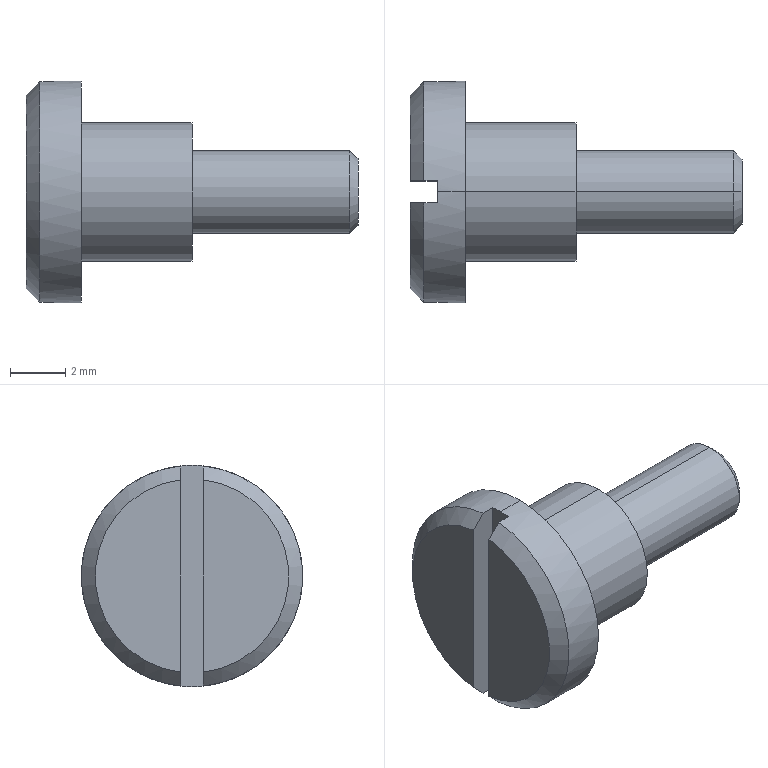Part | STEP file | 0246_012_CBD5-4 | 1 solid | 18 faces | box 12 x 8 x 8 mm | volume 211.87 mm3 | plane 8 | cylinder 6 | cone 4 | commonest cylinder face diameters 3 x2 5 x2 8 x2
STEP:
#1=CARTESIAN_POINT('',(0.,0.,0.));
#2=DIRECTION('',(0.,0.,1.));
#3=DIRECTION('',(1.,0.,0.));
#4=AXIS2_PLACEMENT_3D('',#1,#2,#3);
#5=CARTESIAN_POINT('',(0.,0.,-2.5));
#6=VERTEX_POINT('',#5);
#7=CARTESIAN_POINT('',(0.,0.,2.5));
#8=VERTEX_POINT('',#7);
#9=CARTESIAN_POINT('',(0.,0.,0.));
#10=DIRECTION('',(1.,0.,0.));
#11=DIRECTION('',(0.,0.,-1.));
#12=AXIS2_PLACEMENT_3D('',#9,#10,#11);
#13=CIRCLE('',#12,2.5);
#14=CARTESIAN_POINT('',(2.,0.,0.));
#15=DIRECTION('',(1.,0.,0.));
#16=DIRECTION('',(0.,0.,-1.));
#17=AXIS2_PLACEMENT_3D('',#14,#15,#16);
#18=CYLINDRICAL_SURFACE('',#17,2.5);
#19=CARTESIAN_POINT('',(0.,-2.));
#20=DIRECTION('',(1.,0.));
#21=VECTOR('',#20,1.);
#22=LINE('',#19,#21);
#23=(GEOMETRIC_REPRESENTATION_CONTEXT(2)PARAMETRIC_REPRESENTATION_CONTEXT()REPRESENTATION_CONTEXT('',''));
#24=DEFINITIONAL_REPRESENTATION('',(#22),#23);
#25=PCURVE('',#18,#24);
#26=CARTESIAN_POINT('',(0.,3.25,0.));
#27=DIRECTION('',(1.,0.,0.));
#28=DIRECTION('',(0.,0.,-1.));
#29=AXIS2_PLACEMENT_3D('',#26,#27,#28);
#30=PLANE('',#29);
#31=CARTESIAN_POINT('',(0.,-3.25));
#32=DIRECTION('',(1.,0.));
#33=AXIS2_PLACEMENT_2D('',#31,#32);
#34=CIRCLE('',#33,2.5);
#35=(GEOMETRIC_REPRESENTATION_CONTEXT(2)PARAMETRIC_REPRESENTATION_CONTEXT()REPRESENTATION_CONTEXT('',''));
#36=DEFINITIONAL_REPRESENTATION('',(#34),#35);
#37=PCURVE('',#30,#36);
#38=SURFACE_CURVE('',#13,(#25,#37),.PCURVE_S1.);
#39=EDGE_CURVE('',#6,#8,#38,.T.);
#40=ORIENTED_EDGE('',*,*,#39,.T.);
#41=CARTESIAN_POINT('',(4.,0.,2.5));
#42=VERTEX_POINT('',#41);
#43=CARTESIAN_POINT('',(2.,0.,2.5));
#44=DIRECTION('',(1.,0.,0.));
#45=VECTOR('',#44,1.);
#46=LINE('',#43,#45);
#47=CARTESIAN_POINT('',(3.142,0.));
#48=DIRECTION('',(0.,1.));
#49=VECTOR('',#48,1.);
#50=LINE('',#47,#49);
#51=(GEOMETRIC_REPRESENTATION_CONTEXT(2)PARAMETRIC_REPRESENTATION_CONTEXT()REPRESENTATION_CONTEXT('',''));
#52=DEFINITIONAL_REPRESENTATION('',(#50),#51);
#53=PCURVE('',#18,#52);
#54=CARTESIAN_POINT('',(2.,0.,0.));
#55=DIRECTION('',(1.,0.,0.));
#56=DIRECTION('',(0.,0.,-1.));
#57=AXIS2_PLACEMENT_3D('',#54,#55,#56);
#58=CYLINDRICAL_SURFACE('',#57,2.5);
#59=CARTESIAN_POINT('',(3.142,0.));
#60=DIRECTION('',(0.,1.));
#61=VECTOR('',#60,1.);
#62=LINE('',#59,#61);
#63=(GEOMETRIC_REPRESENTATION_CONTEXT(2)PARAMETRIC_REPRESENTATION_CONTEXT()REPRESENTATION_CONTEXT('',''));
#64=DEFINITIONAL_REPRESENTATION('',(#62),#63);
#65=PCURVE('',#58,#64);
#66=SURFACE_CURVE('',#46,(#53,#65),.PCURVE_S1.);
#67=EDGE_CURVE('',#8,#42,#66,.T.);
#68=ORIENTED_EDGE('',*,*,#67,.T.);
#69=CARTESIAN_POINT('',(4.,0.,-2.5));
#70=VERTEX_POINT('',#69);
#71=CARTESIAN_POINT('',(4.,0.,0.));
#72=DIRECTION('',(-1.,0.,0.));
#73=DIRECTION('',(0.,0.,-1.));
#74=AXIS2_PLACEMENT_3D('',#71,#72,#73);
#75=CIRCLE('',#74,2.5);
#76=CARTESIAN_POINT('',(6.283,2.));
#77=DIRECTION('',(-1.,0.));
#78=VECTOR('',#77,1.);
#79=LINE('',#76,#78);
#80=(GEOMETRIC_REPRESENTATION_CONTEXT(2)PARAMETRIC_REPRESENTATION_CONTEXT()REPRESENTATION_CONTEXT('',''));
#81=DEFINITIONAL_REPRESENTATION('',(#79),#80);
#82=PCURVE('',#18,#81);
#83=CARTESIAN_POINT('',(4.,2.,0.));
#84=DIRECTION('',(1.,0.,0.));
#85=DIRECTION('',(0.,0.,-1.));
#86=AXIS2_PLACEMENT_3D('',#83,#84,#85);
#87=PLANE('',#86);
#88=CARTESIAN_POINT('',(2.5,-2.));
#89=CARTESIAN_POINT('',(2.5,-6.33));
#90=CARTESIAN_POINT('',(-1.25,-4.165));
#91=CARTESIAN_POINT('',(-5.,-2.));
#92=CARTESIAN_POINT('',(-1.25,0.1651));
#93=CARTESIAN_POINT('',(2.5,2.33));
#94=CARTESIAN_POINT('',(2.5,-2.));
#95=(BOUNDED_CURVE()B_SPLINE_CURVE(2,(#88,#89,#90,#91,#92,#93,#94),.UNSPECIFIED.,.T.,.F.)B_SPLINE_CURVE_WITH_KNOTS((1,2,2,2,2,1),(-2.094,0.,2.094,4.189,6.283,8.378),.UNSPECIFIED.)CURVE()GEOMETRIC_REPRESENTATION_ITEM()RATIONAL_B_SPLINE_CURVE((1.,0.5,1.,0.5,1.,0.5,1.))REPRESENTATION_ITEM(''));
#96=(GEOMETRIC_REPRESENTATION_CONTEXT(2)PARAMETRIC_REPRESENTATION_CONTEXT()REPRESENTATION_CONTEXT('',''));
#97=DEFINITIONAL_REPRESENTATION('',(#95),#96);
#98=PCURVE('',#87,#97);
#99=SURFACE_CURVE('',#75,(#82,#98),.PCURVE_S1.);
#100=EDGE_CURVE('',#42,#70,#99,.T.);
#101=ORIENTED_EDGE('',*,*,#100,.T.);
#102=CARTESIAN_POINT('',(2.,0.,-2.5));
#103=DIRECTION('',(1.,0.,0.));
#104=VECTOR('',#103,1.);
#105=LINE('',#102,#104);
#106=CARTESIAN_POINT('',(0.,0.));
#107=DIRECTION('',(0.,1.));
#108=VECTOR('',#107,1.);
#109=LINE('',#106,#108);
#110=(GEOMETRIC_REPRESENTATION_CONTEXT(2)PARAMETRIC_REPRESENTATION_CONTEXT()REPRESENTATION_CONTEXT('',''));
#111=DEFINITIONAL_REPRESENTATION('',(#109),#110);
#112=PCURVE('',#18,#111);
#113=CARTESIAN_POINT('',(6.283,0.));
#114=DIRECTION('',(0.,1.));
#115=VECTOR('',#114,1.);
#116=LINE('',#113,#115);
#117=(GEOMETRIC_REPRESENTATION_CONTEXT(2)PARAMETRIC_REPRESENTATION_CONTEXT()REPRESENTATION_CONTEXT('',''));
#118=DEFINITIONAL_REPRESENTATION('',(#116),#117);
#119=PCURVE('',#58,#118);
#120=SURFACE_CURVE('',#105,(#112,#119),.PCURVE_S1.);
#121=EDGE_CURVE('',#6,#70,#120,.T.);
#122=ORIENTED_EDGE('',*,*,#121,.F.);
#123=EDGE_LOOP('',(#40,#68,#101,#122));
#124=FACE_BOUND('',#123,.T.);
#125=ADVANCED_FACE('',(#124),#18,.T.);
#126=CARTESIAN_POINT('',(-1.,0.4,3.98));
#127=VERTEX_POINT('',#126);
#128=CARTESIAN_POINT('',(-1.,0.,4.));
#129=VERTEX_POINT('',#128);
#130=CARTESIAN_POINT('',(-1.,0.,0.));
#131=DIRECTION('',(1.,0.,0.));
#132=DIRECTION('',(0.,0.,-1.));
#133=AXIS2_PLACEMENT_3D('',#130,#131,#132);
#134=CIRCLE('',#133,4.);
#135=CARTESIAN_POINT('',(-0.75,0.,0.));
#136=DIRECTION('',(1.,0.,0.));
#137=DIRECTION('',(0.,0.,-1.));
#138=AXIS2_PLACEMENT_3D('',#135,#136,#137);
#139=CYLINDRICAL_SURFACE('',#138,4.);
#140=CARTESIAN_POINT('',(0.,-0.25));
#141=DIRECTION('',(1.,0.));
#142=VECTOR('',#141,1.);
#143=LINE('',#140,#142);
#144=(GEOMETRIC_REPRESENTATION_CONTEXT(2)PARAMETRIC_REPRESENTATION_CONTEXT()REPRESENTATION_CONTEXT('',''));
#145=DEFINITIONAL_REPRESENTATION('',(#143),#144);
#146=PCURVE('',#139,#145);
#147=CARTESIAN_POINT('',(-1.,-0.4,5.6));
#148=DIRECTION('',(1.,0.,0.));
#149=DIRECTION('',(0.,0.,-1.));
#150=AXIS2_PLACEMENT_3D('',#147,#148,#149);
#151=PLANE('',#150);
#152=CARTESIAN_POINT('',(5.6,0.4));
#153=DIRECTION('',(1.,0.));
#154=AXIS2_PLACEMENT_2D('',#152,#153);
#155=CIRCLE('',#154,4.);
#156=(GEOMETRIC_REPRESENTATION_CONTEXT(2)PARAMETRIC_REPRESENTATION_CONTEXT()REPRESENTATION_CONTEXT('',''));
#157=DEFINITIONAL_REPRESENTATION('',(#155),#156);
#158=PCURVE('',#151,#157);
#159=SURFACE_CURVE('',#134,(#146,#158),.PCURVE_S1.);
#160=EDGE_CURVE('',#127,#129,#159,.T.);
#161=ORIENTED_EDGE('',*,*,#160,.T.);
#162=CARTESIAN_POINT('',(0.,0.,4.));
#163=VERTEX_POINT('',#162);
#164=CARTESIAN_POINT('',(-0.75,0.,4.));
#165=DIRECTION('',(1.,0.,0.));
#166=VECTOR('',#165,1.);
#167=LINE('',#164,#166);
#168=CARTESIAN_POINT('',(3.142,0.));
#169=DIRECTION('',(0.,1.));
#170=VECTOR('',#169,1.);
#171=LINE('',#168,#170);
#172=(GEOMETRIC_REPRESENTATION_CONTEXT(2)PARAMETRIC_REPRESENTATION_CONTEXT()REPRESENTATION_CONTEXT('',''));
#173=DEFINITIONAL_REPRESENTATION('',(#171),#172);
#174=PCURVE('',#139,#173);
#175=CARTESIAN_POINT('',(-0.75,0.,0.));
#176=DIRECTION('',(1.,0.,0.));
#177=DIRECTION('',(0.,0.,-1.));
#178=AXIS2_PLACEMENT_3D('',#175,#176,#177);
#179=CYLINDRICAL_SURFACE('',#178,4.);
#180=CARTESIAN_POINT('',(3.142,0.));
#181=DIRECTION('',(0.,1.));
#182=VECTOR('',#181,1.);
#183=LINE('',#180,#182);
#184=(GEOMETRIC_REPRESENTATION_CONTEXT(2)PARAMETRIC_REPRESENTATION_CONTEXT()REPRESENTATION_CONTEXT('',''));
#185=DEFINITIONAL_REPRESENTATION('',(#183),#184);
#186=PCURVE('',#179,#185);
#187=SURFACE_CURVE('',#167,(#174,#186),.PCURVE_S1.);
#188=EDGE_CURVE('',#129,#163,#187,.T.);
#189=ORIENTED_EDGE('',*,*,#188,.T.);
#190=CARTESIAN_POINT('',(0.,0.,-4.));
#191=VERTEX_POINT('',#190);
#192=CARTESIAN_POINT('',(0.,0.,0.));
#193=DIRECTION('',(1.,0.,0.));
#194=DIRECTION('',(0.,0.,-1.));
#195=AXIS2_PLACEMENT_3D('',#192,#193,#194);
#196=CIRCLE('',#195,4.);
#197=CARTESIAN_POINT('',(0.,0.75));
#198=DIRECTION('',(1.,0.));
#199=VECTOR('',#198,1.);
#200=LINE('',#197,#199);
#201=(GEOMETRIC_REPRESENTATION_CONTEXT(2)PARAMETRIC_REPRESENTATION_CONTEXT()REPRESENTATION_CONTEXT('',''));
#202=DEFINITIONAL_REPRESENTATION('',(#200),#201);
#203=PCURVE('',#139,#202);
#204=CARTESIAN_POINT('',(0.,-3.25));
#205=DIRECTION('',(1.,0.));
#206=AXIS2_PLACEMENT_2D('',#204,#205);
#207=CIRCLE('',#206,4.);
#208=(GEOMETRIC_REPRESENTATION_CONTEXT(2)PARAMETRIC_REPRESENTATION_CONTEXT()REPRESENTATION_CONTEXT('',''));
#209=DEFINITIONAL_REPRESENTATION('',(#207),#208);
#210=PCURVE('',#30,#209);
#211=SURFACE_CURVE('',#196,(#203,#210),.PCURVE_S1.);
#212=EDGE_CURVE('',#191,#163,#211,.T.);
#213=ORIENTED_EDGE('',*,*,#212,.F.);
#214=CARTESIAN_POINT('',(-1.,0.,-4.));
#215=VERTEX_POINT('',#214);
#216=CARTESIAN_POINT('',(-0.75,0.,-4.));
#217=DIRECTION('',(1.,0.,0.));
#218=VECTOR('',#217,1.);
#219=LINE('',#216,#218);
#220=CARTESIAN_POINT('',(0.,0.));
#221=DIRECTION('',(0.,1.));
#222=VECTOR('',#221,1.);
#223=LINE('',#220,#222);
#224=(GEOMETRIC_REPRESENTATION_CONTEXT(2)PARAMETRIC_REPRESENTATION_CONTEXT()REPRESENTATION_CONTEXT('',''));
#225=DEFINITIONAL_REPRESENTATION('',(#223),#224);
#226=PCURVE('',#139,#225);
#227=CARTESIAN_POINT('',(6.283,0.));
#228=DIRECTION('',(0.,1.));
#229=VECTOR('',#228,1.);
#230=LINE('',#227,#229);
#231=(GEOMETRIC_REPRESENTATION_CONTEXT(2)PARAMETRIC_REPRESENTATION_CONTEXT()REPRESENTATION_CONTEXT('',''));
#232=DEFINITIONAL_REPRESENTATION('',(#230),#231);
#233=PCURVE('',#179,#232);
#234=SURFACE_CURVE('',#219,(#226,#233),.PCURVE_S1.);
#235=EDGE_CURVE('',#215,#191,#234,.T.);
#236=ORIENTED_EDGE('',*,*,#235,.F.);
#237=CARTESIAN_POINT('',(-1.,0.4,-3.98));
#238=VERTEX_POINT('',#237);
#239=CARTESIAN_POINT('',(-1.,0.,0.));
#240=DIRECTION('',(1.,0.,0.));
#241=DIRECTION('',(0.,0.,-1.));
#242=AXIS2_PLACEMENT_3D('',#239,#240,#241);
#243=CIRCLE('',#242,4.);
#244=CARTESIAN_POINT('',(0.,-0.25));
#245=DIRECTION('',(1.,0.));
#246=VECTOR('',#245,1.);
#247=LINE('',#244,#246);
#248=(GEOMETRIC_REPRESENTATION_CONTEXT(2)PARAMETRIC_REPRESENTATION_CONTEXT()REPRESENTATION_CONTEXT('',''));
#249=DEFINITIONAL_REPRESENTATION('',(#247),#248);
#250=PCURVE('',#139,#249);
#251=CARTESIAN_POINT('',(5.6,0.4));
#252=DIRECTION('',(1.,0.));
#253=AXIS2_PLACEMENT_2D('',#251,#252);
#254=CIRCLE('',#253,4.);
#255=(GEOMETRIC_REPRESENTATION_CONTEXT(2)PARAMETRIC_REPRESENTATION_CONTEXT()REPRESENTATION_CONTEXT('',''));
#256=DEFINITIONAL_REPRESENTATION('',(#254),#255);
#257=PCURVE('',#151,#256);
#258=SURFACE_CURVE('',#243,(#250,#257),.PCURVE_S1.);
#259=EDGE_CURVE('',#215,#238,#258,.T.);
#260=ORIENTED_EDGE('',*,*,#259,.T.);
#261=CARTESIAN_POINT('',(-1.5,0.4,-3.98));
#262=VERTEX_POINT('',#261);
#263=CARTESIAN_POINT('',(-1.,0.4,-3.98));
#264=DIRECTION('',(-1.,0.,0.));
#265=VECTOR('',#264,1.);
#266=LINE('',#263,#265);
#267=CARTESIAN_POINT('',(0.1002,-0.25));
#268=DIRECTION('',(0.,-1.));
#269=VECTOR('',#268,1.);
#270=LINE('',#267,#269);
#271=(GEOMETRIC_REPRESENTATION_CONTEXT(2)PARAMETRIC_REPRESENTATION_CONTEXT()REPRESENTATION_CONTEXT('',''));
#272=DEFINITIONAL_REPRESENTATION('',(#270),#271);
#273=PCURVE('',#139,#272);
#274=CARTESIAN_POINT('',(-1.,0.4,5.6));
#275=DIRECTION('',(0.,1.,0.));
#276=DIRECTION('',(0.,0.,1.));
#277=AXIS2_PLACEMENT_3D('',#274,#275,#276);
#278=PLANE('',#277);
#279=CARTESIAN_POINT('',(-9.58,0.));
#280=DIRECTION('',(0.,-1.));
#281=VECTOR('',#280,1.);
#282=LINE('',#279,#281);
#283=(GEOMETRIC_REPRESENTATION_CONTEXT(2)PARAMETRIC_REPRESENTATION_CONTEXT()REPRESENTATION_CONTEXT('',''));
#284=DEFINITIONAL_REPRESENTATION('',(#282),#283);
#285=PCURVE('',#278,#284);
#286=SURFACE_CURVE('',#266,(#273,#285),.PCURVE_S1.);
#287=EDGE_CURVE('',#238,#262,#286,.T.);
#288=ORIENTED_EDGE('',*,*,#287,.T.);
#289=CARTESIAN_POINT('',(-1.5,0.4,3.98));
#290=VERTEX_POINT('',#289);
#291=CARTESIAN_POINT('',(-1.5,0.,0.));
#292=DIRECTION('',(1.,0.,0.));
#293=DIRECTION('',(0.,0.,-1.));
#294=AXIS2_PLACEMENT_3D('',#291,#292,#293);
#295=CIRCLE('',#294,4.);
#296=CARTESIAN_POINT('',(0.,-0.75));
#297=DIRECTION('',(1.,0.));
#298=VECTOR('',#297,1.);
#299=LINE('',#296,#298);
#300=(GEOMETRIC_REPRESENTATION_CONTEXT(2)PARAMETRIC_REPRESENTATION_CONTEXT()REPRESENTATION_CONTEXT('',''));
#301=DEFINITIONAL_REPRESENTATION('',(#299),#300);
#302=PCURVE('',#139,#301);
#303=CARTESIAN_POINT('',(-1.5,0.,0.));
#304=DIRECTION('',(1.,0.,0.));
#305=DIRECTION('',(0.,0.,-1.));
#306=AXIS2_PLACEMENT_3D('',#303,#304,#305);
#307=CONICAL_SURFACE('',#306,4.,0.7854);
#308=CARTESIAN_POINT('',(0.,0.));
#309=DIRECTION('',(1.,0.));
#310=VECTOR('',#309,1.);
#311=LINE('',#308,#310);
#312=(GEOMETRIC_REPRESENTATION_CONTEXT(2)PARAMETRIC_REPRESENTATION_CONTEXT()REPRESENTATION_CONTEXT('',''));
#313=DEFINITIONAL_REPRESENTATION('',(#311),#312);
#314=PCURVE('',#307,#313);
#315=SURFACE_CURVE('',#295,(#302,#314),.PCURVE_S1.);
#316=EDGE_CURVE('',#262,#290,#315,.T.);
#317=ORIENTED_EDGE('',*,*,#316,.T.);
#318=CARTESIAN_POINT('',(-1.,0.4,3.98));
#319=DIRECTION('',(1.,0.,0.));
#320=VECTOR('',#319,1.);
#321=LINE('',#318,#320);
#322=CARTESIAN_POINT('',(3.041,-0.25));
#323=DIRECTION('',(0.,1.));
#324=VECTOR('',#323,1.);
#325=LINE('',#322,#324);
#326=(GEOMETRIC_REPRESENTATION_CONTEXT(2)PARAMETRIC_REPRESENTATION_CONTEXT()REPRESENTATION_CONTEXT('',''));
#327=DEFINITIONAL_REPRESENTATION('',(#325),#326);
#328=PCURVE('',#139,#327);
#329=CARTESIAN_POINT('',(-1.62,0.));
#330=DIRECTION('',(0.,1.));
#331=VECTOR('',#330,1.);
#332=LINE('',#329,#331);
#333=(GEOMETRIC_REPRESENTATION_CONTEXT(2)PARAMETRIC_REPRESENTATION_CONTEXT()REPRESENTATION_CONTEXT('',''));
#334=DEFINITIONAL_REPRESENTATION('',(#332),#333);
#335=PCURVE('',#278,#334);
#336=SURFACE_CURVE('',#321,(#328,#335),.PCURVE_S1.);
#337=EDGE_CURVE('',#290,#127,#336,.T.);
#338=ORIENTED_EDGE('',*,*,#337,.T.);
#339=EDGE_LOOP('',(#161,#189,#213,#236,#260,#288,#317,#338));
#340=FACE_BOUND('',#339,.T.);
#341=ADVANCED_FACE('',(#340),#139,.T.);
#342=CARTESIAN_POINT('',(4.,0.,1.5));
#343=VERTEX_POINT('',#342);
#344=CARTESIAN_POINT('',(4.,0.,-1.5));
#345=VERTEX_POINT('',#344);
#346=CARTESIAN_POINT('',(4.,0.,0.));
#347=DIRECTION('',(-1.,0.,0.));
#348=DIRECTION('',(0.,0.,-1.));
#349=AXIS2_PLACEMENT_3D('',#346,#347,#348);
#350=CIRCLE('',#349,1.5);
#351=CARTESIAN_POINT('',(6.847,0.,0.));
#352=DIRECTION('',(1.,0.,0.));
#353=DIRECTION('',(0.,0.,-1.));
#354=AXIS2_PLACEMENT_3D('',#351,#352,#353);
#355=CYLINDRICAL_SURFACE('',#354,1.5);
#356=CARTESIAN_POINT('',(6.283,-2.847));
#357=DIRECTION('',(-1.,0.));
#358=VECTOR('',#357,1.);
#359=LINE('',#356,#358);
#360=(GEOMETRIC_REPRESENTATION_CONTEXT(2)PARAMETRIC_REPRESENTATION_CONTEXT()REPRESENTATION_CONTEXT('',''));
#361=DEFINITIONAL_REPRESENTATION('',(#359),#360);
#362=PCURVE('',#355,#361);
#363=CARTESIAN_POINT('',(1.5,-2.));
#364=CARTESIAN_POINT('',(1.5,-4.598));
#365=CARTESIAN_POINT('',(-0.75,-3.299));
#366=CARTESIAN_POINT('',(-3.,-2.));
#367=CARTESIAN_POINT('',(-0.75,-0.701));
#368=CARTESIAN_POINT('',(1.5,0.5981));
#369=CARTESIAN_POINT('',(1.5,-2.));
#370=(BOUNDED_CURVE()B_SPLINE_CURVE(2,(#363,#364,#365,#366,#367,#368,#369),.UNSPECIFIED.,.T.,.F.)B_SPLINE_CURVE_WITH_KNOTS((1,2,2,2,2,1),(-2.094,0.,2.094,4.189,6.283,8.378),.UNSPECIFIED.)CURVE()GEOMETRIC_REPRESENTATION_ITEM()RATIONAL_B_SPLINE_CURVE((1.,0.5,1.,0.5,1.,0.5,1.))REPRESENTATION_ITEM(''));
#371=(GEOMETRIC_REPRESENTATION_CONTEXT(2)PARAMETRIC_REPRESENTATION_CONTEXT()REPRESENTATION_CONTEXT('',''));
#372=DEFINITIONAL_REPRESENTATION('',(#370),#371);
#373=PCURVE('',#87,#372);
#374=SURFACE_CURVE('',#350,(#362,#373),.PCURVE_S1.);
#375=EDGE_CURVE('',#343,#345,#374,.T.);
#376=ORIENTED_EDGE('',*,*,#375,.F.);
#377=CARTESIAN_POINT('',(9.694,0.,1.5));
#378=VERTEX_POINT('',#377);
#379=CARTESIAN_POINT('',(6.847,0.,1.5));
#380=DIRECTION('',(1.,0.,0.));
#381=VECTOR('',#380,1.);
#382=LINE('',#379,#381);
#383=CARTESIAN_POINT('',(3.142,0.));
#384=DIRECTION('',(0.,1.));
#385=VECTOR('',#384,1.);
#386=LINE('',#383,#385);
#387=(GEOMETRIC_REPRESENTATION_CONTEXT(2)PARAMETRIC_REPRESENTATION_CONTEXT()REPRESENTATION_CONTEXT('',''));
#388=DEFINITIONAL_REPRESENTATION('',(#386),#387);
#389=PCURVE('',#355,#388);
#390=CARTESIAN_POINT('',(6.847,0.,0.));
#391=DIRECTION('',(1.,0.,0.));
#392=DIRECTION('',(0.,0.,-1.));
#393=AXIS2_PLACEMENT_3D('',#390,#391,#392);
#394=CYLINDRICAL_SURFACE('',#393,1.5);
#395=CARTESIAN_POINT('',(3.142,0.));
#396=DIRECTION('',(0.,1.));
#397=VECTOR('',#396,1.);
#398=LINE('',#395,#397);
#399=(GEOMETRIC_REPRESENTATION_CONTEXT(2)PARAMETRIC_REPRESENTATION_CONTEXT()REPRESENTATION_CONTEXT('',''));
#400=DEFINITIONAL_REPRESENTATION('',(#398),#399);
#401=PCURVE('',#394,#400);
#402=SURFACE_CURVE('',#382,(#389,#401),.PCURVE_S1.);
#403=EDGE_CURVE('',#343,#378,#402,.T.);
#404=ORIENTED_EDGE('',*,*,#403,.T.);
#405=CARTESIAN_POINT('',(9.694,0.,-1.5));
#406=VERTEX_POINT('',#405);
#407=CARTESIAN_POINT('',(9.694,0.,0.));
#408=DIRECTION('',(-1.,0.,0.));
#409=DIRECTION('',(0.,0.,-1.));
#410=AXIS2_PLACEMENT_3D('',#407,#408,#409);
#411=CIRCLE('',#410,1.5);
#412=CARTESIAN_POINT('',(6.283,2.847));
#413=DIRECTION('',(-1.,0.));
#414=VECTOR('',#413,1.);
#415=LINE('',#412,#414);
#416=(GEOMETRIC_REPRESENTATION_CONTEXT(2)PARAMETRIC_REPRESENTATION_CONTEXT()REPRESENTATION_CONTEXT('',''));
#417=DEFINITIONAL_REPRESENTATION('',(#415),#416);
#418=PCURVE('',#355,#417);
#419=CARTESIAN_POINT('',(9.694,0.,0.));
#420=DIRECTION('',(-1.,0.,0.));
#421=DIRECTION('',(0.,0.,1.));
#422=AXIS2_PLACEMENT_3D('',#419,#420,#421);
#423=CONICAL_SURFACE('',#422,1.5,0.7854);
#424=CARTESIAN_POINT('',(-3.142,0.));
#425=DIRECTION('',(1.,0.));
#426=VECTOR('',#425,1.);
#427=LINE('',#424,#426);
#428=(GEOMETRIC_REPRESENTATION_CONTEXT(2)PARAMETRIC_REPRESENTATION_CONTEXT()REPRESENTATION_CONTEXT('',''));
#429=DEFINITIONAL_REPRESENTATION('',(#427),#428);
#430=PCURVE('',#423,#429);
#431=SURFACE_CURVE('',#411,(#418,#430),.PCURVE_S1.);
#432=EDGE_CURVE('',#378,#406,#431,.T.);
#433=ORIENTED_EDGE('',*,*,#432,.T.);
#434=CARTESIAN_POINT('',(6.847,0.,-1.5));
#435=DIRECTION('',(1.,0.,0.));
#436=VECTOR('',#435,1.);
#437=LINE('',#434,#436);
#438=CARTESIAN_POINT('',(0.,0.));
#439=DIRECTION('',(0.,1.));
#440=VECTOR('',#439,1.);
#441=LINE('',#438,#440);
#442=(GEOMETRIC_REPRESENTATION_CONTEXT(2)PARAMETRIC_REPRESENTATION_CONTEXT()REPRESENTATION_CONTEXT('',''));
#443=DEFINITIONAL_REPRESENTATION('',(#441),#442);
#444=PCURVE('',#355,#443);
#445=CARTESIAN_POINT('',(6.283,0.));
#446=DIRECTION('',(0.,1.));
#447=VECTOR('',#446,1.);
#448=LINE('',#445,#447);
#449=(GEOMETRIC_REPRESENTATION_CONTEXT(2)PARAMETRIC_REPRESENTATION_CONTEXT()REPRESENTATION_CONTEXT('',''));
#450=DEFINITIONAL_REPRESENTATION('',(#448),#449);
#451=PCURVE('',#394,#450);
#452=SURFACE_CURVE('',#437,(#444,#451),.PCURVE_S1.);
#453=EDGE_CURVE('',#345,#406,#452,.T.);
#454=ORIENTED_EDGE('',*,*,#453,.F.);
#455=EDGE_LOOP('',(#376,#404,#433,#454));
#456=FACE_BOUND('',#455,.T.);
#457=ADVANCED_FACE('',(#456),#355,.T.);
#458=CARTESIAN_POINT('',(10.,0.,1.194));
#459=VERTEX_POINT('',#458);
#460=CARTESIAN_POINT('',(10.,0.,-1.194));
#461=VERTEX_POINT('',#460);
#462=CARTESIAN_POINT('',(10.,0.,0.));
#463=DIRECTION('',(-1.,0.,0.));
#464=DIRECTION('',(0.,0.,1.));
#465=AXIS2_PLACEMENT_3D('',#462,#463,#464);
#466=CIRCLE('',#465,1.194);
#467=CARTESIAN_POINT('',(0.,-0.3065));
#468=DIRECTION('',(1.,0.));
#469=VECTOR('',#468,1.);
#470=LINE('',#467,#469);
#471=(GEOMETRIC_REPRESENTATION_CONTEXT(2)PARAMETRIC_REPRESENTATION_CONTEXT()REPRESENTATION_CONTEXT('',''));
#472=DEFINITIONAL_REPRESENTATION('',(#470),#471);
#473=PCURVE('',#423,#472);
#474=CARTESIAN_POINT('',(10.,0.5968,0.));
#475=DIRECTION('',(1.,0.,0.));
#476=DIRECTION('',(0.,0.,-1.));
#477=AXIS2_PLACEMENT_3D('',#474,#475,#476);
#478=PLANE('',#477);
#479=CARTESIAN_POINT('',(-1.194,-0.5968));
#480=CARTESIAN_POINT('',(-1.194,1.47));
#481=CARTESIAN_POINT('',(0.5968,0.4369));
#482=CARTESIAN_POINT('',(2.387,-0.5968));
#483=CARTESIAN_POINT('',(0.5968,-1.63));
#484=CARTESIAN_POINT('',(-1.194,-2.664));
#485=CARTESIAN_POINT('',(-1.194,-0.5968));
#486=(BOUNDED_CURVE()B_SPLINE_CURVE(2,(#479,#480,#481,#482,#483,#484,#485),.UNSPECIFIED.,.T.,.F.)B_SPLINE_CURVE_WITH_KNOTS((1,2,2,2,2,1),(-2.094,0.,2.094,4.189,6.283,8.378),.UNSPECIFIED.)CURVE()GEOMETRIC_REPRESENTATION_ITEM()RATIONAL_B_SPLINE_CURVE((1.,0.5,1.,0.5,1.,0.5,1.))REPRESENTATION_ITEM(''));
#487=(GEOMETRIC_REPRESENTATION_CONTEXT(2)PARAMETRIC_REPRESENTATION_CONTEXT()REPRESENTATION_CONTEXT('',''));
#488=DEFINITIONAL_REPRESENTATION('',(#486),#487);
#489=PCURVE('',#478,#488);
#490=SURFACE_CURVE('',#466,(#473,#489),.PCURVE_S1.);
#491=EDGE_CURVE('',#459,#461,#490,.T.);
#492=ORIENTED_EDGE('',*,*,#491,.T.);
#493=CARTESIAN_POINT('',(9.694,0.,-1.5));
#494=DIRECTION('',(-0.7071,0.,-0.7071));
#495=VECTOR('',#494,1.);
#496=LINE('',#493,#495);
#497=CARTESIAN_POINT('',(3.142,0.));
#498=DIRECTION('',(0.,1.));
#499=VECTOR('',#498,1.);
#500=LINE('',#497,#499);
#501=(GEOMETRIC_REPRESENTATION_CONTEXT(2)PARAMETRIC_REPRESENTATION_CONTEXT()REPRESENTATION_CONTEXT('',''));
#502=DEFINITIONAL_REPRESENTATION('',(#500),#501);
#503=PCURVE('',#423,#502);
#504=CARTESIAN_POINT('',(9.694,0.,0.));
#505=DIRECTION('',(-1.,0.,0.));
#506=DIRECTION('',(0.,0.,1.));
#507=AXIS2_PLACEMENT_3D('',#504,#505,#506);
#508=CONICAL_SURFACE('',#507,1.5,0.7854);
#509=CARTESIAN_POINT('',(3.142,0.));
#510=DIRECTION('',(0.,1.));
#511=VECTOR('',#510,1.);
#512=LINE('',#509,#511);
#513=(GEOMETRIC_REPRESENTATION_CONTEXT(2)PARAMETRIC_REPRESENTATION_CONTEXT()REPRESENTATION_CONTEXT('',''));
#514=DEFINITIONAL_REPRESENTATION('',(#512),#513);
#515=PCURVE('',#508,#514);
#516=SURFACE_CURVE('',#496,(#503,#515),.PCURVE_S1.);
#517=EDGE_CURVE('',#461,#406,#516,.T.);
#518=ORIENTED_EDGE('',*,*,#517,.T.);
#519=ORIENTED_EDGE('',*,*,#432,.F.);
#520=CARTESIAN_POINT('',(9.694,0.,1.5));
#521=DIRECTION('',(-0.7071,0.,0.7071));
#522=VECTOR('',#521,1.);
#523=LINE('',#520,#522);
#524=CARTESIAN_POINT('',(0.,0.));
#525=DIRECTION('',(0.,1.));
#526=VECTOR('',#525,1.);
#527=LINE('',#524,#526);
#528=(GEOMETRIC_REPRESENTATION_CONTEXT(2)PARAMETRIC_REPRESENTATION_CONTEXT()REPRESENTATION_CONTEXT('',''));
#529=DEFINITIONAL_REPRESENTATION('',(#527),#528);
#530=PCURVE('',#423,#529);
#531=CARTESIAN_POINT('',(6.283,0.));
#532=DIRECTION('',(0.,1.));
#533=VECTOR('',#532,1.);
#534=LINE('',#531,#533);
#535=(GEOMETRIC_REPRESENTATION_CONTEXT(2)PARAMETRIC_REPRESENTATION_CONTEXT()REPRESENTATION_CONTEXT('',''));
#536=DEFINITIONAL_REPRESENTATION('',(#534),#535);
#537=PCURVE('',#508,#536);
#538=SURFACE_CURVE('',#523,(#530,#537),.PCURVE_S1.);
#539=EDGE_CURVE('',#459,#378,#538,.T.);
#540=ORIENTED_EDGE('',*,*,#539,.F.);
#541=EDGE_LOOP('',(#492,#518,#519,#540));
#542=FACE_BOUND('',#541,.T.);
#543=ADVANCED_FACE('',(#542),#423,.T.);
#544=ORIENTED_EDGE('',*,*,#67,.F.);
#545=CARTESIAN_POINT('',(0.,0.,0.));
#546=DIRECTION('',(1.,0.,0.));
#547=DIRECTION('',(0.,0.,-1.));
#548=AXIS2_PLACEMENT_3D('',#545,#546,#547);
#549=CIRCLE('',#548,2.5);
#550=CARTESIAN_POINT('',(0.,-2.));
#551=DIRECTION('',(1.,0.));
#552=VECTOR('',#551,1.);
#553=LINE('',#550,#552);
#554=(GEOMETRIC_REPRESENTATION_CONTEXT(2)PARAMETRIC_REPRESENTATION_CONTEXT()REPRESENTATION_CONTEXT('',''));
#555=DEFINITIONAL_REPRESENTATION('',(#553),#554);
#556=PCURVE('',#58,#555);
#557=CARTESIAN_POINT('',(0.,-3.25));
#558=DIRECTION('',(1.,0.));
#559=AXIS2_PLACEMENT_2D('',#557,#558);
#560=CIRCLE('',#559,2.5);
#561=(GEOMETRIC_REPRESENTATION_CONTEXT(2)PARAMETRIC_REPRESENTATION_CONTEXT()REPRESENTATION_CONTEXT('',''));
#562=DEFINITIONAL_REPRESENTATION('',(#560),#561);
#563=PCURVE('',#30,#562);
#564=SURFACE_CURVE('',#549,(#556,#563),.PCURVE_S1.);
#565=EDGE_CURVE('',#8,#6,#564,.T.);
#566=ORIENTED_EDGE('',*,*,#565,.T.);
#567=ORIENTED_EDGE('',*,*,#121,.T.);
#568=CARTESIAN_POINT('',(4.,0.,0.));
#569=DIRECTION('',(-1.,0.,0.));
#570=DIRECTION('',(0.,0.,-1.));
#571=AXIS2_PLACEMENT_3D('',#568,#569,#570);
#572=CIRCLE('',#571,2.5);
#573=CARTESIAN_POINT('',(6.283,2.));
#574=DIRECTION('',(-1.,0.));
#575=VECTOR('',#574,1.);
#576=LINE('',#573,#575);
#577=(GEOMETRIC_REPRESENTATION_CONTEXT(2)PARAMETRIC_REPRESENTATION_CONTEXT()REPRESENTATION_CONTEXT('',''));
#578=DEFINITIONAL_REPRESENTATION('',(#576),#577);
#579=PCURVE('',#58,#578);
#580=CARTESIAN_POINT('',(2.5,-2.));
#581=CARTESIAN_POINT('',(2.5,-6.33));
#582=CARTESIAN_POINT('',(-1.25,-4.165));
#583=CARTESIAN_POINT('',(-5.,-2.));
#584=CARTESIAN_POINT('',(-1.25,0.1651));
#585=CARTESIAN_POINT('',(2.5,2.33));
#586=CARTESIAN_POINT('',(2.5,-2.));
#587=(BOUNDED_CURVE()B_SPLINE_CURVE(2,(#580,#581,#582,#583,#584,#585,#586),.UNSPECIFIED.,.T.,.F.)B_SPLINE_CURVE_WITH_KNOTS((1,2,2,2,2,1),(-2.094,0.,2.094,4.189,6.283,8.378),.UNSPECIFIED.)CURVE()GEOMETRIC_REPRESENTATION_ITEM()RATIONAL_B_SPLINE_CURVE((1.,0.5,1.,0.5,1.,0.5,1.))REPRESENTATION_ITEM(''));
#588=(GEOMETRIC_REPRESENTATION_CONTEXT(2)PARAMETRIC_REPRESENTATION_CONTEXT()REPRESENTATION_CONTEXT('',''));
#589=DEFINITIONAL_REPRESENTATION('',(#587),#588);
#590=PCURVE('',#87,#589);
#591=SURFACE_CURVE('',#572,(#579,#590),.PCURVE_S1.);
#592=EDGE_CURVE('',#70,#42,#591,.T.);
#593=ORIENTED_EDGE('',*,*,#592,.T.);
#594=EDGE_LOOP('',(#544,#566,#567,#593));
#595=FACE_BOUND('',#594,.T.);
#596=ADVANCED_FACE('',(#595),#58,.T.);
#597=ORIENTED_EDGE('',*,*,#39,.F.);
#598=ORIENTED_EDGE('',*,*,#565,.F.);
#599=EDGE_LOOP('',(#597,#598));
#600=FACE_BOUND('',#599,.T.);
#601=ORIENTED_EDGE('',*,*,#212,.T.);
#602=CARTESIAN_POINT('',(0.,0.,0.));
#603=DIRECTION('',(1.,0.,0.));
#604=DIRECTION('',(0.,0.,-1.));
#605=AXIS2_PLACEMENT_3D('',#602,#603,#604);
#606=CIRCLE('',#605,4.);
#607=CARTESIAN_POINT('',(0.,-3.25));
#608=DIRECTION('',(1.,0.));
#609=AXIS2_PLACEMENT_2D('',#607,#608);
#610=CIRCLE('',#609,4.);
#611=(GEOMETRIC_REPRESENTATION_CONTEXT(2)PARAMETRIC_REPRESENTATION_CONTEXT()REPRESENTATION_CONTEXT('',''));
#612=DEFINITIONAL_REPRESENTATION('',(#610),#611);
#613=PCURVE('',#30,#612);
#614=CARTESIAN_POINT('',(0.,0.75));
#615=DIRECTION('',(1.,0.));
#616=VECTOR('',#615,1.);
#617=LINE('',#614,#616);
#618=(GEOMETRIC_REPRESENTATION_CONTEXT(2)PARAMETRIC_REPRESENTATION_CONTEXT()REPRESENTATION_CONTEXT('',''));
#619=DEFINITIONAL_REPRESENTATION('',(#617),#618);
#620=PCURVE('',#179,#619);
#621=SURFACE_CURVE('',#606,(#613,#620),.PCURVE_S1.);
#622=EDGE_CURVE('',#163,#191,#621,.T.);
#623=ORIENTED_EDGE('',*,*,#622,.T.);
#624=EDGE_LOOP('',(#601,#623));
#625=FACE_BOUND('',#624,.T.);
#626=ADVANCED_FACE('',(#600,#625),#30,.T.);
#627=CARTESIAN_POINT('',(4.,0.,0.));
#628=DIRECTION('',(-1.,0.,0.));
#629=DIRECTION('',(0.,0.,-1.));
#630=AXIS2_PLACEMENT_3D('',#627,#628,#629);
#631=CIRCLE('',#630,1.5);
#632=CARTESIAN_POINT('',(1.5,-2.));
#633=CARTESIAN_POINT('',(1.5,-4.598));
#634=CARTESIAN_POINT('',(-0.75,-3.299));
#635=CARTESIAN_POINT('',(-3.,-2.));
#636=CARTESIAN_POINT('',(-0.75,-0.701));
#637=CARTESIAN_POINT('',(1.5,0.5981));
#638=CARTESIAN_POINT('',(1.5,-2.));
#639=(BOUNDED_CURVE()B_SPLINE_CURVE(2,(#632,#633,#634,#635,#636,#637,#638),.UNSPECIFIED.,.T.,.F.)B_SPLINE_CURVE_WITH_KNOTS((1,2,2,2,2,1),(-2.094,0.,2.094,4.189,6.283,8.378),.UNSPECIFIED.)CURVE()GEOMETRIC_REPRESENTATION_ITEM()RATIONAL_B_SPLINE_CURVE((1.,0.5,1.,0.5,1.,0.5,1.))REPRESENTATION_ITEM(''));
#640=(GEOMETRIC_REPRESENTATION_CONTEXT(2)PARAMETRIC_REPRESENTATION_CONTEXT()REPRESENTATION_CONTEXT('',''));
#641=DEFINITIONAL_REPRESENTATION('',(#639),#640);
#642=PCURVE('',#87,#641);
#643=CARTESIAN_POINT('',(6.283,-2.847));
#644=DIRECTION('',(-1.,0.));
#645=VECTOR('',#644,1.);
#646=LINE('',#643,#645);
#647=(GEOMETRIC_REPRESENTATION_CONTEXT(2)PARAMETRIC_REPRESENTATION_CONTEXT()REPRESENTATION_CONTEXT('',''));
#648=DEFINITIONAL_REPRESENTATION('',(#646),#647);
#649=PCURVE('',#394,#648);
#650=SURFACE_CURVE('',#631,(#642,#649),.PCURVE_S1.);
#651=EDGE_CURVE('',#345,#343,#650,.T.);
#652=ORIENTED_EDGE('',*,*,#651,.T.);
#653=ORIENTED_EDGE('',*,*,#375,.T.);
#654=EDGE_LOOP('',(#652,#653));
#655=FACE_BOUND('',#654,.T.);
#656=ORIENTED_EDGE('',*,*,#592,.F.);
#657=ORIENTED_EDGE('',*,*,#100,.F.);
#658=EDGE_LOOP('',(#656,#657));
#659=FACE_BOUND('',#658,.T.);
#660=ADVANCED_FACE('',(#655,#659),#87,.T.);
#661=ORIENTED_EDGE('',*,*,#188,.F.);
#662=CARTESIAN_POINT('',(-1.,-0.4,3.98));
#663=VERTEX_POINT('',#662);
#664=CARTESIAN_POINT('',(-1.,0.,0.));
#665=DIRECTION('',(1.,0.,0.));
#666=DIRECTION('',(0.,0.,-1.));
#667=AXIS2_PLACEMENT_3D('',#664,#665,#666);
#668=CIRCLE('',#667,4.);
#669=CARTESIAN_POINT('',(0.,-0.25));
#670=DIRECTION('',(1.,0.));
#671=VECTOR('',#670,1.);
#672=LINE('',#669,#671);
#673=(GEOMETRIC_REPRESENTATION_CONTEXT(2)PARAMETRIC_REPRESENTATION_CONTEXT()REPRESENTATION_CONTEXT('',''));
#674=DEFINITIONAL_REPRESENTATION('',(#672),#673);
#675=PCURVE('',#179,#674);
#676=CARTESIAN_POINT('',(5.6,0.4));
#677=DIRECTION('',(1.,0.));
#678=AXIS2_PLACEMENT_2D('',#676,#677);
#679=CIRCLE('',#678,4.);
#680=(GEOMETRIC_REPRESENTATION_CONTEXT(2)PARAMETRIC_REPRESENTATION_CONTEXT()REPRESENTATION_CONTEXT('',''));
#681=DEFINITIONAL_REPRESENTATION('',(#679),#680);
#682=PCURVE('',#151,#681);
#683=SURFACE_CURVE('',#668,(#675,#682),.PCURVE_S1.);
#684=EDGE_CURVE('',#129,#663,#683,.T.);
#685=ORIENTED_EDGE('',*,*,#684,.T.);
#686=CARTESIAN_POINT('',(-1.5,-0.4,3.98));
#687=VERTEX_POINT('',#686);
#688=CARTESIAN_POINT('',(-3.,-0.4,3.98));
#689=DIRECTION('',(-1.,0.,0.));
#690=VECTOR('',#689,1.);
#691=LINE('',#688,#690);
#692=CARTESIAN_POINT('',(3.242,-2.25));
#693=DIRECTION('',(0.,-1.));
#694=VECTOR('',#693,1.);
#695=LINE('',#692,#694);
#696=(GEOMETRIC_REPRESENTATION_CONTEXT(2)PARAMETRIC_REPRESENTATION_CONTEXT()REPRESENTATION_CONTEXT('',''));
#697=DEFINITIONAL_REPRESENTATION('',(#695),#696);
#698=PCURVE('',#179,#697);
#699=CARTESIAN_POINT('',(-3.,-0.4,5.6));
#700=DIRECTION('',(0.,-1.,0.));
#701=DIRECTION('',(0.,0.,-1.));
#702=AXIS2_PLACEMENT_3D('',#699,#700,#701);
#703=PLANE('',#702);
#704=CARTESIAN_POINT('',(1.62,0.));
#705=DIRECTION('',(0.,-1.));
#706=VECTOR('',#705,1.);
#707=LINE('',#704,#706);
#708=(GEOMETRIC_REPRESENTATION_CONTEXT(2)PARAMETRIC_REPRESENTATION_CONTEXT()REPRESENTATION_CONTEXT('',''));
#709=DEFINITIONAL_REPRESENTATION('',(#707),#708);
#710=PCURVE('',#703,#709);
#711=SURFACE_CURVE('',#691,(#698,#710),.PCURVE_S1.);
#712=EDGE_CURVE('',#663,#687,#711,.T.);
#713=ORIENTED_EDGE('',*,*,#712,.T.);
#714=CARTESIAN_POINT('',(-1.5,-0.4,-3.98));
#715=VERTEX_POINT('',#714);
#716=CARTESIAN_POINT('',(-1.5,0.,0.));
#717=DIRECTION('',(1.,0.,0.));
#718=DIRECTION('',(0.,0.,-1.));
#719=AXIS2_PLACEMENT_3D('',#716,#717,#718);
#720=CIRCLE('',#719,4.);
#721=CARTESIAN_POINT('',(0.,-0.75));
#722=DIRECTION('',(1.,0.));
#723=VECTOR('',#722,1.);
#724=LINE('',#721,#723);
#725=(GEOMETRIC_REPRESENTATION_CONTEXT(2)PARAMETRIC_REPRESENTATION_CONTEXT()REPRESENTATION_CONTEXT('',''));
#726=DEFINITIONAL_REPRESENTATION('',(#724),#725);
#727=PCURVE('',#179,#726);
#728=CARTESIAN_POINT('',(-1.5,0.,0.));
#729=DIRECTION('',(1.,0.,0.));
#730=DIRECTION('',(0.,0.,-1.));
#731=AXIS2_PLACEMENT_3D('',#728,#729,#730);
#732=CONICAL_SURFACE('',#731,4.,0.7854);
#733=CARTESIAN_POINT('',(0.,0.));
#734=DIRECTION('',(1.,0.));
#735=VECTOR('',#734,1.);
#736=LINE('',#733,#735);
#737=(GEOMETRIC_REPRESENTATION_CONTEXT(2)PARAMETRIC_REPRESENTATION_CONTEXT()REPRESENTATION_CONTEXT('',''));
#738=DEFINITIONAL_REPRESENTATION('',(#736),#737);
#739=PCURVE('',#732,#738);
#740=SURFACE_CURVE('',#720,(#727,#739),.PCURVE_S1.);
#741=EDGE_CURVE('',#687,#715,#740,.T.);
#742=ORIENTED_EDGE('',*,*,#741,.T.);
#743=CARTESIAN_POINT('',(-1.,-0.4,-3.98));
#744=VERTEX_POINT('',#743);
#745=CARTESIAN_POINT('',(-3.,-0.4,-3.98));
#746=DIRECTION('',(1.,0.,0.));
#747=VECTOR('',#746,1.);
#748=LINE('',#745,#747);
#749=CARTESIAN_POINT('',(6.183,-2.25));
#750=DIRECTION('',(0.,1.));
#751=VECTOR('',#750,1.);
#752=LINE('',#749,#751);
#753=(GEOMETRIC_REPRESENTATION_CONTEXT(2)PARAMETRIC_REPRESENTATION_CONTEXT()REPRESENTATION_CONTEXT('',''));
#754=DEFINITIONAL_REPRESENTATION('',(#752),#753);
#755=PCURVE('',#179,#754);
#756=CARTESIAN_POINT('',(9.58,0.));
#757=DIRECTION('',(0.,1.));
#758=VECTOR('',#757,1.);
#759=LINE('',#756,#758);
#760=(GEOMETRIC_REPRESENTATION_CONTEXT(2)PARAMETRIC_REPRESENTATION_CONTEXT()REPRESENTATION_CONTEXT('',''));
#761=DEFINITIONAL_REPRESENTATION('',(#759),#760);
#762=PCURVE('',#703,#761);
#763=SURFACE_CURVE('',#748,(#755,#762),.PCURVE_S1.);
#764=EDGE_CURVE('',#715,#744,#763,.T.);
#765=ORIENTED_EDGE('',*,*,#764,.T.);
#766=CARTESIAN_POINT('',(-1.,0.,0.));
#767=DIRECTION('',(1.,0.,0.));
#768=DIRECTION('',(0.,0.,-1.));
#769=AXIS2_PLACEMENT_3D('',#766,#767,#768);
#770=CIRCLE('',#769,4.);
#771=CARTESIAN_POINT('',(0.,-0.25));
#772=DIRECTION('',(1.,0.));
#773=VECTOR('',#772,1.);
#774=LINE('',#771,#773);
#775=(GEOMETRIC_REPRESENTATION_CONTEXT(2)PARAMETRIC_REPRESENTATION_CONTEXT()REPRESENTATION_CONTEXT('',''));
#776=DEFINITIONAL_REPRESENTATION('',(#774),#775);
#777=PCURVE('',#179,#776);
#778=CARTESIAN_POINT('',(5.6,0.4));
#779=DIRECTION('',(1.,0.));
#780=AXIS2_PLACEMENT_2D('',#778,#779);
#781=CIRCLE('',#780,4.);
#782=(GEOMETRIC_REPRESENTATION_CONTEXT(2)PARAMETRIC_REPRESENTATION_CONTEXT()REPRESENTATION_CONTEXT('',''));
#783=DEFINITIONAL_REPRESENTATION('',(#781),#782);
#784=PCURVE('',#151,#783);
#785=SURFACE_CURVE('',#770,(#777,#784),.PCURVE_S1.);
#786=EDGE_CURVE('',#744,#215,#785,.T.);
#787=ORIENTED_EDGE('',*,*,#786,.T.);
#788=ORIENTED_EDGE('',*,*,#235,.T.);
#789=ORIENTED_EDGE('',*,*,#622,.F.);
#790=EDGE_LOOP('',(#661,#685,#713,#742,#765,#787,#788,#789));
#791=FACE_BOUND('',#790,.T.);
#792=ADVANCED_FACE('',(#791),#179,.T.);
#793=ORIENTED_EDGE('',*,*,#403,.F.);
#794=ORIENTED_EDGE('',*,*,#651,.F.);
#795=ORIENTED_EDGE('',*,*,#453,.T.);
#796=CARTESIAN_POINT('',(9.694,0.,0.));
#797=DIRECTION('',(-1.,0.,0.));
#798=DIRECTION('',(0.,0.,-1.));
#799=AXIS2_PLACEMENT_3D('',#796,#797,#798);
#800=CIRCLE('',#799,1.5);
#801=CARTESIAN_POINT('',(6.283,2.847));
#802=DIRECTION('',(-1.,0.));
#803=VECTOR('',#802,1.);
#804=LINE('',#801,#803);
#805=(GEOMETRIC_REPRESENTATION_CONTEXT(2)PARAMETRIC_REPRESENTATION_CONTEXT()REPRESENTATION_CONTEXT('',''));
#806=DEFINITIONAL_REPRESENTATION('',(#804),#805);
#807=PCURVE('',#394,#806);
#808=CARTESIAN_POINT('',(3.142,0.));
#809=DIRECTION('',(1.,0.));
#810=VECTOR('',#809,1.);
#811=LINE('',#808,#810);
#812=(GEOMETRIC_REPRESENTATION_CONTEXT(2)PARAMETRIC_REPRESENTATION_CONTEXT()REPRESENTATION_CONTEXT('',''));
#813=DEFINITIONAL_REPRESENTATION('',(#811),#812);
#814=PCURVE('',#508,#813);
#815=SURFACE_CURVE('',#800,(#807,#814),.PCURVE_S1.);
#816=EDGE_CURVE('',#406,#378,#815,.T.);
#817=ORIENTED_EDGE('',*,*,#816,.T.);
#818=EDGE_LOOP('',(#793,#794,#795,#817));
#819=FACE_BOUND('',#818,.T.);
#820=ADVANCED_FACE('',(#819),#394,.T.);
#821=CARTESIAN_POINT('',(-2.,-0.4,3.477));
#822=VERTEX_POINT('',#821);
#823=CARTESIAN_POINT('',(-1.5,-0.4,3.98));
#824=CARTESIAN_POINT('',(-1.667,-0.4,3.812));
#825=CARTESIAN_POINT('',(-1.833,-0.4,3.645));
#826=CARTESIAN_POINT('',(-2.,-0.4,3.477));
#827=B_SPLINE_CURVE_WITH_KNOTS('',3,(#823,#824,#825,#826),.UNSPECIFIED.,.F.,.F.,(4,4),(0.,0.0007091),.PIECEWISE_BEZIER_KNOTS.);
#828=CARTESIAN_POINT('',(3.242,0.));
#829=CARTESIAN_POINT('',(3.242,-0.007579));
#830=CARTESIAN_POINT('',(3.242,-0.02274));
#831=CARTESIAN_POINT('',(3.243,-0.04547));
#832=CARTESIAN_POINT('',(3.244,-0.0682));
#833=CARTESIAN_POINT('',(3.244,-0.09094));
#834=CARTESIAN_POINT('',(3.245,-0.1137));
#835=CARTESIAN_POINT('',(3.245,-0.1364));
#836=CARTESIAN_POINT('',(3.246,-0.1591));
#837=CARTESIAN_POINT('',(3.247,-0.1819));
#838=CARTESIAN_POINT('',(3.247,-0.2046));
#839=CARTESIAN_POINT('',(3.248,-0.2273));
#840=CARTESIAN_POINT('',(3.248,-0.25));
#841=CARTESIAN_POINT('',(3.249,-0.2728));
#842=CARTESIAN_POINT('',(3.25,-0.2955));
#843=CARTESIAN_POINT('',(3.25,-0.3182));
#844=CARTESIAN_POINT('',(3.251,-0.341));
#845=CARTESIAN_POINT('',(3.252,-0.3637));
#846=CARTESIAN_POINT('',(3.253,-0.3864));
#847=CARTESIAN_POINT('',(3.253,-0.4091));
#848=CARTESIAN_POINT('',(3.254,-0.4318));
#849=CARTESIAN_POINT('',(3.255,-0.4546));
#850=CARTESIAN_POINT('',(3.255,-0.4773));
#851=CARTESIAN_POINT('',(3.256,-0.4924));
#852=CARTESIAN_POINT('',(3.256,-0.5));
#853=B_SPLINE_CURVE_WITH_KNOTS('',3,(#828,#829,#830,#831,#832,#833,#834,#835,#836,#837,#838,#839,#840,#841,#842,#843,#844,#845,#846,#847,#848,#849,#850,#851,#852),.UNSPECIFIED.,.F.,.F.,(4,1,1,1,1,1,1,1,1,1,1,1,1,1,1,1,1,1,1,1,1,1,4),(0.,0.00003223,0.00006447,0.0000967,0.0001289,0.0001612,0.0001934,0.0002256,0.0002579,0.0002901,0.0003223,0.0003546,0.0003868,0.000419,0.0004513,0.0004835,0.0005157,0.000548,0.0005802,0.0006124,0.0006447,0.0006769,0.0007091),.QUASI_UNIFORM_KNOTS.);
#854=(GEOMETRIC_REPRESENTATION_CONTEXT(2)PARAMETRIC_REPRESENTATION_CONTEXT()REPRESENTATION_CONTEXT('',''));
#855=DEFINITIONAL_REPRESENTATION('',(#853),#854);
#856=PCURVE('',#732,#855);
#857=CARTESIAN_POINT('',(1.62,1.5));
#858=CARTESIAN_POINT('',(1.788,1.333));
#859=CARTESIAN_POINT('',(1.955,1.167));
#860=CARTESIAN_POINT('',(2.123,1.));
#861=B_SPLINE_CURVE_WITH_KNOTS('',3,(#857,#858,#859,#860),.UNSPECIFIED.,.F.,.F.,(4,4),(0.,0.0007091),.PIECEWISE_BEZIER_KNOTS.);
#862=(GEOMETRIC_REPRESENTATION_CONTEXT(2)PARAMETRIC_REPRESENTATION_CONTEXT()REPRESENTATION_CONTEXT('',''));
#863=DEFINITIONAL_REPRESENTATION('',(#861),#862);
#864=PCURVE('',#703,#863);
#865=SURFACE_CURVE('',#827,(#856,#864),.PCURVE_S1.);
#866=EDGE_CURVE('',#687,#822,#865,.T.);
#867=ORIENTED_EDGE('',*,*,#866,.T.);
#868=CARTESIAN_POINT('',(-2.,-0.4,-3.477));
#869=VERTEX_POINT('',#868);
#870=CARTESIAN_POINT('',(-2.,0.,0.));
#871=DIRECTION('',(1.,0.,0.));
#872=DIRECTION('',(0.,0.,-1.));
#873=AXIS2_PLACEMENT_3D('',#870,#871,#872);
#874=CIRCLE('',#873,3.5);
#875=CARTESIAN_POINT('',(0.,-0.5));
#876=DIRECTION('',(1.,0.));
#877=VECTOR('',#876,1.);
#878=LINE('',#875,#877);
#879=(GEOMETRIC_REPRESENTATION_CONTEXT(2)PARAMETRIC_REPRESENTATION_CONTEXT()REPRESENTATION_CONTEXT('',''));
#880=DEFINITIONAL_REPRESENTATION('',(#878),#879);
#881=PCURVE('',#732,#880);
#882=CARTESIAN_POINT('',(-2.,1.75,0.));
#883=DIRECTION('',(-1.,0.,0.));
#884=DIRECTION('',(0.,0.,1.));
#885=AXIS2_PLACEMENT_3D('',#882,#883,#884);
#886=PLANE('',#885);
#887=CARTESIAN_POINT('',(-3.5,-1.75));
#888=CARTESIAN_POINT('',(-3.5,4.312));
#889=CARTESIAN_POINT('',(1.75,1.281));
#890=CARTESIAN_POINT('',(7.,-1.75));
#891=CARTESIAN_POINT('',(1.75,-4.781));
#892=CARTESIAN_POINT('',(-3.5,-7.812));
#893=CARTESIAN_POINT('',(-3.5,-1.75));
#894=(BOUNDED_CURVE()B_SPLINE_CURVE(2,(#887,#888,#889,#890,#891,#892,#893),.UNSPECIFIED.,.T.,.F.)B_SPLINE_CURVE_WITH_KNOTS((1,2,2,2,2,1),(-2.094,0.,2.094,4.189,6.283,8.378),.UNSPECIFIED.)CURVE()GEOMETRIC_REPRESENTATION_ITEM()RATIONAL_B_SPLINE_CURVE((1.,0.5,1.,0.5,1.,0.5,1.))REPRESENTATION_ITEM(''));
#895=(GEOMETRIC_REPRESENTATION_CONTEXT(2)PARAMETRIC_REPRESENTATION_CONTEXT()REPRESENTATION_CONTEXT('',''));
#896=DEFINITIONAL_REPRESENTATION('',(#894),#895);
#897=PCURVE('',#886,#896);
#898=SURFACE_CURVE('',#874,(#881,#897),.PCURVE_S1.);
#899=EDGE_CURVE('',#822,#869,#898,.T.);
#900=ORIENTED_EDGE('',*,*,#899,.T.);
#901=CARTESIAN_POINT('',(-2.,-0.4,-3.477));
#902=CARTESIAN_POINT('',(-1.833,-0.4,-3.645));
#903=CARTESIAN_POINT('',(-1.667,-0.4,-3.812));
#904=CARTESIAN_POINT('',(-1.5,-0.4,-3.98));
#905=B_SPLINE_CURVE_WITH_KNOTS('',3,(#901,#902,#903,#904),.UNSPECIFIED.,.F.,.F.,(4,4),(0.,0.0007091),.PIECEWISE_BEZIER_KNOTS.);
#906=CARTESIAN_POINT('',(6.169,-0.5));
#907=CARTESIAN_POINT('',(6.169,-0.4924));
#908=CARTESIAN_POINT('',(6.169,-0.4773));
#909=CARTESIAN_POINT('',(6.17,-0.4546));
#910=CARTESIAN_POINT('',(6.171,-0.4318));
#911=CARTESIAN_POINT('',(6.172,-0.4091));
#912=CARTESIAN_POINT('',(6.172,-0.3864));
#913=CARTESIAN_POINT('',(6.173,-0.3637));
#914=CARTESIAN_POINT('',(6.174,-0.341));
#915=CARTESIAN_POINT('',(6.174,-0.3182));
#916=CARTESIAN_POINT('',(6.175,-0.2955));
#917=CARTESIAN_POINT('',(6.176,-0.2728));
#918=CARTESIAN_POINT('',(6.176,-0.25));
#919=CARTESIAN_POINT('',(6.177,-0.2273));
#920=CARTESIAN_POINT('',(6.178,-0.2046));
#921=CARTESIAN_POINT('',(6.178,-0.1819));
#922=CARTESIAN_POINT('',(6.179,-0.1591));
#923=CARTESIAN_POINT('',(6.179,-0.1364));
#924=CARTESIAN_POINT('',(6.18,-0.1137));
#925=CARTESIAN_POINT('',(6.181,-0.09094));
#926=CARTESIAN_POINT('',(6.181,-0.0682));
#927=CARTESIAN_POINT('',(6.182,-0.04547));
#928=CARTESIAN_POINT('',(6.182,-0.02274));
#929=CARTESIAN_POINT('',(6.183,-0.007579));
#930=CARTESIAN_POINT('',(6.183,0.));
#931=B_SPLINE_CURVE_WITH_KNOTS('',3,(#906,#907,#908,#909,#910,#911,#912,#913,#914,#915,#916,#917,#918,#919,#920,#921,#922,#923,#924,#925,#926,#927,#928,#929,#930),.UNSPECIFIED.,.F.,.F.,(4,1,1,1,1,1,1,1,1,1,1,1,1,1,1,1,1,1,1,1,1,1,4),(0.,0.00003223,0.00006447,0.0000967,0.0001289,0.0001612,0.0001934,0.0002256,0.0002579,0.0002901,0.0003223,0.0003546,0.0003868,0.000419,0.0004513,0.0004835,0.0005157,0.000548,0.0005802,0.0006124,0.0006447,0.0006769,0.0007091),.QUASI_UNIFORM_KNOTS.);
#932=(GEOMETRIC_REPRESENTATION_CONTEXT(2)PARAMETRIC_REPRESENTATION_CONTEXT()REPRESENTATION_CONTEXT('',''));
#933=DEFINITIONAL_REPRESENTATION('',(#931),#932);
#934=PCURVE('',#732,#933);
#935=CARTESIAN_POINT('',(9.077,1.));
#936=CARTESIAN_POINT('',(9.245,1.167));
#937=CARTESIAN_POINT('',(9.412,1.333));
#938=CARTESIAN_POINT('',(9.58,1.5));
#939=B_SPLINE_CURVE_WITH_KNOTS('',3,(#935,#936,#937,#938),.UNSPECIFIED.,.F.,.F.,(4,4),(0.,0.0007091),.PIECEWISE_BEZIER_KNOTS.);
#940=(GEOMETRIC_REPRESENTATION_CONTEXT(2)PARAMETRIC_REPRESENTATION_CONTEXT()REPRESENTATION_CONTEXT('',''));
#941=DEFINITIONAL_REPRESENTATION('',(#939),#940);
#942=PCURVE('',#703,#941);
#943=SURFACE_CURVE('',#905,(#934,#942),.PCURVE_S1.);
#944=EDGE_CURVE('',#869,#715,#943,.T.);
#945=ORIENTED_EDGE('',*,*,#944,.T.);
#946=ORIENTED_EDGE('',*,*,#741,.F.);
#947=EDGE_LOOP('',(#867,#900,#945,#946));
#948=FACE_BOUND('',#947,.T.);
#949=ADVANCED_FACE('',(#948),#732,.T.);
#950=CARTESIAN_POINT('',(-2.,0.4,3.477));
#951=VERTEX_POINT('',#950);
#952=CARTESIAN_POINT('',(-2.,0.4,3.477));
#953=CARTESIAN_POINT('',(-1.833,0.4,3.645));
#954=CARTESIAN_POINT('',(-1.667,0.4,3.812));
#955=CARTESIAN_POINT('',(-1.5,0.4,3.98));
#956=B_SPLINE_CURVE_WITH_KNOTS('',3,(#952,#953,#954,#955),.UNSPECIFIED.,.F.,.F.,(4,4),(0.,0.0007091),.PIECEWISE_BEZIER_KNOTS.);
#957=CARTESIAN_POINT('',(3.027,-0.5));
#958=CARTESIAN_POINT('',(3.027,-0.4924));
#959=CARTESIAN_POINT('',(3.028,-0.4773));
#960=CARTESIAN_POINT('',(3.029,-0.4546));
#961=CARTESIAN_POINT('',(3.029,-0.4318));
#962=CARTESIAN_POINT('',(3.03,-0.4091));
#963=CARTESIAN_POINT('',(3.031,-0.3864));
#964=CARTESIAN_POINT('',(3.031,-0.3637));
#965=CARTESIAN_POINT('',(3.032,-0.341));
#966=CARTESIAN_POINT('',(3.033,-0.3182));
#967=CARTESIAN_POINT('',(3.033,-0.2955));
#968=CARTESIAN_POINT('',(3.034,-0.2728));
#969=CARTESIAN_POINT('',(3.035,-0.25));
#970=CARTESIAN_POINT('',(3.035,-0.2273));
#971=CARTESIAN_POINT('',(3.036,-0.2046));
#972=CARTESIAN_POINT('',(3.037,-0.1819));
#973=CARTESIAN_POINT('',(3.037,-0.1591));
#974=CARTESIAN_POINT('',(3.038,-0.1364));
#975=CARTESIAN_POINT('',(3.038,-0.1137));
#976=CARTESIAN_POINT('',(3.039,-0.09094));
#977=CARTESIAN_POINT('',(3.04,-0.0682));
#978=CARTESIAN_POINT('',(3.04,-0.04547));
#979=CARTESIAN_POINT('',(3.041,-0.02274));
#980=CARTESIAN_POINT('',(3.041,-0.007579));
#981=CARTESIAN_POINT('',(3.041,0.));
#982=B_SPLINE_CURVE_WITH_KNOTS('',3,(#957,#958,#959,#960,#961,#962,#963,#964,#965,#966,#967,#968,#969,#970,#971,#972,#973,#974,#975,#976,#977,#978,#979,#980,#981),.UNSPECIFIED.,.F.,.F.,(4,1,1,1,1,1,1,1,1,1,1,1,1,1,1,1,1,1,1,1,1,1,4),(0.,0.00003223,0.00006447,0.0000967,0.0001289,0.0001612,0.0001934,0.0002256,0.0002579,0.0002901,0.0003223,0.0003546,0.0003868,0.000419,0.0004513,0.0004835,0.0005157,0.000548,0.0005802,0.0006124,0.0006447,0.0006769,0.0007091),.QUASI_UNIFORM_KNOTS.);
#983=(GEOMETRIC_REPRESENTATION_CONTEXT(2)PARAMETRIC_REPRESENTATION_CONTEXT()REPRESENTATION_CONTEXT('',''));
#984=DEFINITIONAL_REPRESENTATION('',(#982),#983);
#985=PCURVE('',#307,#984);
#986=CARTESIAN_POINT('',(-2.123,-1.));
#987=CARTESIAN_POINT('',(-1.955,-0.8334));
#988=CARTESIAN_POINT('',(-1.788,-0.6667));
#989=CARTESIAN_POINT('',(-1.62,-0.5));
#990=B_SPLINE_CURVE_WITH_KNOTS('',3,(#986,#987,#988,#989),.UNSPECIFIED.,.F.,.F.,(4,4),(0.,0.0007091),.PIECEWISE_BEZIER_KNOTS.);
#991=(GEOMETRIC_REPRESENTATION_CONTEXT(2)PARAMETRIC_REPRESENTATION_CONTEXT()REPRESENTATION_CONTEXT('',''));
#992=DEFINITIONAL_REPRESENTATION('',(#990),#991);
#993=PCURVE('',#278,#992);
#994=SURFACE_CURVE('',#956,(#985,#993),.PCURVE_S1.);
#995=EDGE_CURVE('',#951,#290,#994,.T.);
#996=ORIENTED_EDGE('',*,*,#995,.T.);
#997=ORIENTED_EDGE('',*,*,#316,.F.);
#998=CARTESIAN_POINT('',(-2.,0.4,-3.477));
#999=VERTEX_POINT('',#998);
#1000=CARTESIAN_POINT('',(-1.5,0.4,-3.98));
#1001=CARTESIAN_POINT('',(-1.667,0.4,-3.812));
#1002=CARTESIAN_POINT('',(-1.833,0.4,-3.645));
#1003=CARTESIAN_POINT('',(-2.,0.4,-3.477));
#1004=B_SPLINE_CURVE_WITH_KNOTS('',3,(#1000,#1001,#1002,#1003),.UNSPECIFIED.,.F.,.F.,(4,4),(0.,0.0007091),.PIECEWISE_BEZIER_KNOTS.);
#1005=CARTESIAN_POINT('',(0.1002,0.));
#1006=CARTESIAN_POINT('',(0.1004,-0.007579));
#1007=CARTESIAN_POINT('',(0.1007,-0.02274));
#1008=CARTESIAN_POINT('',(0.1013,-0.04547));
#1009=CARTESIAN_POINT('',(0.1019,-0.0682));
#1010=CARTESIAN_POINT('',(0.1025,-0.09094));
#1011=CARTESIAN_POINT('',(0.1031,-0.1137));
#1012=CARTESIAN_POINT('',(0.1037,-0.1364));
#1013=CARTESIAN_POINT('',(0.1043,-0.1591));
#1014=CARTESIAN_POINT('',(0.105,-0.1819));
#1015=CARTESIAN_POINT('',(0.1056,-0.2046));
#1016=CARTESIAN_POINT('',(0.1062,-0.2273));
#1017=CARTESIAN_POINT('',(0.1069,-0.25));
#1018=CARTESIAN_POINT('',(0.1075,-0.2728));
#1019=CARTESIAN_POINT('',(0.1082,-0.2955));
#1020=CARTESIAN_POINT('',(0.1089,-0.3182));
#1021=CARTESIAN_POINT('',(0.1095,-0.341));
#1022=CARTESIAN_POINT('',(0.1102,-0.3637));
#1023=CARTESIAN_POINT('',(0.1109,-0.3864));
#1024=CARTESIAN_POINT('',(0.1116,-0.4091));
#1025=CARTESIAN_POINT('',(0.1123,-0.4318));
#1026=CARTESIAN_POINT('',(0.1131,-0.4546));
#1027=CARTESIAN_POINT('',(0.1138,-0.4773));
#1028=CARTESIAN_POINT('',(0.1143,-0.4924));
#1029=CARTESIAN_POINT('',(0.1145,-0.5));
#1030=B_SPLINE_CURVE_WITH_KNOTS('',3,(#1005,#1006,#1007,#1008,#1009,#1010,#1011,#1012,#1013,#1014,#1015,#1016,#1017,#1018,#1019,#1020,#1021,#1022,#1023,#1024,#1025,#1026,#1027,#1028,#1029),.UNSPECIFIED.,.F.,.F.,(4,1,1,1,1,1,1,1,1,1,1,1,1,1,1,1,1,1,1,1,1,1,4),(0.,0.00003223,0.00006447,0.0000967,0.0001289,0.0001612,0.0001934,0.0002256,0.0002579,0.0002901,0.0003223,0.0003546,0.0003868,0.000419,0.0004513,0.0004835,0.0005157,0.000548,0.0005802,0.0006124,0.0006447,0.0006769,0.0007091),.QUASI_UNIFORM_KNOTS.);
#1031=(GEOMETRIC_REPRESENTATION_CONTEXT(2)PARAMETRIC_REPRESENTATION_CONTEXT()REPRESENTATION_CONTEXT('',''));
#1032=DEFINITIONAL_REPRESENTATION('',(#1030),#1031);
#1033=PCURVE('',#307,#1032);
#1034=CARTESIAN_POINT('',(-9.58,-0.5));
#1035=CARTESIAN_POINT('',(-9.412,-0.6667));
#1036=CARTESIAN_POINT('',(-9.245,-0.8334));
#1037=CARTESIAN_POINT('',(-9.077,-1.));
#1038=B_SPLINE_CURVE_WITH_KNOTS('',3,(#1034,#1035,#1036,#1037),.UNSPECIFIED.,.F.,.F.,(4,4),(0.,0.0007091),.PIECEWISE_BEZIER_KNOTS.);
#1039=(GEOMETRIC_REPRESENTATION_CONTEXT(2)PARAMETRIC_REPRESENTATION_CONTEXT()REPRESENTATION_CONTEXT('',''));
#1040=DEFINITIONAL_REPRESENTATION('',(#1038),#1039);
#1041=PCURVE('',#278,#1040);
#1042=SURFACE_CURVE('',#1004,(#1033,#1041),.PCURVE_S1.);
#1043=EDGE_CURVE('',#262,#999,#1042,.T.);
#1044=ORIENTED_EDGE('',*,*,#1043,.T.);
#1045=CARTESIAN_POINT('',(-2.,0.,0.));
#1046=DIRECTION('',(1.,0.,0.));
#1047=DIRECTION('',(0.,0.,-1.));
#1048=AXIS2_PLACEMENT_3D('',#1045,#1046,#1047);
#1049=CIRCLE('',#1048,3.5);
#1050=CARTESIAN_POINT('',(0.,-0.5));
#1051=DIRECTION('',(1.,0.));
#1052=VECTOR('',#1051,1.);
#1053=LINE('',#1050,#1052);
#1054=(GEOMETRIC_REPRESENTATION_CONTEXT(2)PARAMETRIC_REPRESENTATION_CONTEXT()REPRESENTATION_CONTEXT('',''));
#1055=DEFINITIONAL_REPRESENTATION('',(#1053),#1054);
#1056=PCURVE('',#307,#1055);
#1057=CARTESIAN_POINT('',(-2.,1.75,0.));
#1058=DIRECTION('',(-1.,0.,0.));
#1059=DIRECTION('',(0.,0.,1.));
#1060=AXIS2_PLACEMENT_3D('',#1057,#1058,#1059);
#1061=PLANE('',#1060);
#1062=CARTESIAN_POINT('',(-3.5,-1.75));
#1063=CARTESIAN_POINT('',(-3.5,4.312));
#1064=CARTESIAN_POINT('',(1.75,1.281));
#1065=CARTESIAN_POINT('',(7.,-1.75));
#1066=CARTESIAN_POINT('',(1.75,-4.781));
#1067=CARTESIAN_POINT('',(-3.5,-7.812));
#1068=CARTESIAN_POINT('',(-3.5,-1.75));
#1069=(BOUNDED_CURVE()B_SPLINE_CURVE(2,(#1062,#1063,#1064,#1065,#1066,#1067,#1068),.UNSPECIFIED.,.T.,.F.)B_SPLINE_CURVE_WITH_KNOTS((1,2,2,2,2,1),(-2.094,0.,2.094,4.189,6.283,8.378),.UNSPECIFIED.)CURVE()GEOMETRIC_REPRESENTATION_ITEM()RATIONAL_B_SPLINE_CURVE((1.,0.5,1.,0.5,1.,0.5,1.))REPRESENTATION_ITEM(''));
#1070=(GEOMETRIC_REPRESENTATION_CONTEXT(2)PARAMETRIC_REPRESENTATION_CONTEXT()REPRESENTATION_CONTEXT('',''));
#1071=DEFINITIONAL_REPRESENTATION('',(#1069),#1070);
#1072=PCURVE('',#1061,#1071);
#1073=SURFACE_CURVE('',#1049,(#1056,#1072),.PCURVE_S1.);
#1074=EDGE_CURVE('',#999,#951,#1073,.T.);
#1075=ORIENTED_EDGE('',*,*,#1074,.T.);
#1076=EDGE_LOOP('',(#996,#997,#1044,#1075));
#1077=FACE_BOUND('',#1076,.T.);
#1078=ADVANCED_FACE('',(#1077),#307,.T.);
#1079=ORIENTED_EDGE('',*,*,#517,.F.);
#1080=CARTESIAN_POINT('',(10.,0.,0.));
#1081=DIRECTION('',(-1.,0.,0.));
#1082=DIRECTION('',(0.,0.,1.));
#1083=AXIS2_PLACEMENT_3D('',#1080,#1081,#1082);
#1084=CIRCLE('',#1083,1.194);
#1085=CARTESIAN_POINT('',(0.,-0.3065));
#1086=DIRECTION('',(1.,0.));
#1087=VECTOR('',#1086,1.);
#1088=LINE('',#1085,#1087);
#1089=(GEOMETRIC_REPRESENTATION_CONTEXT(2)PARAMETRIC_REPRESENTATION_CONTEXT()REPRESENTATION_CONTEXT('',''));
#1090=DEFINITIONAL_REPRESENTATION('',(#1088),#1089);
#1091=PCURVE('',#508,#1090);
#1092=CARTESIAN_POINT('',(-1.194,-0.5968));
#1093=CARTESIAN_POINT('',(-1.194,1.47));
#1094=CARTESIAN_POINT('',(0.5968,0.4369));
#1095=CARTESIAN_POINT('',(2.387,-0.5968));
#1096=CARTESIAN_POINT('',(0.5968,-1.63));
#1097=CARTESIAN_POINT('',(-1.194,-2.664));
#1098=CARTESIAN_POINT('',(-1.194,-0.5968));
#1099=(BOUNDED_CURVE()B_SPLINE_CURVE(2,(#1092,#1093,#1094,#1095,#1096,#1097,#1098),.UNSPECIFIED.,.T.,.F.)B_SPLINE_CURVE_WITH_KNOTS((1,2,2,2,2,1),(-2.094,0.,2.094,4.189,6.283,8.378),.UNSPECIFIED.)CURVE()GEOMETRIC_REPRESENTATION_ITEM()RATIONAL_B_SPLINE_CURVE((1.,0.5,1.,0.5,1.,0.5,1.))REPRESENTATION_ITEM(''));
#1100=(GEOMETRIC_REPRESENTATION_CONTEXT(2)PARAMETRIC_REPRESENTATION_CONTEXT()REPRESENTATION_CONTEXT('',''));
#1101=DEFINITIONAL_REPRESENTATION('',(#1099),#1100);
#1102=PCURVE('',#478,#1101);
#1103=SURFACE_CURVE('',#1084,(#1091,#1102),.PCURVE_S1.);
#1104=EDGE_CURVE('',#461,#459,#1103,.T.);
#1105=ORIENTED_EDGE('',*,*,#1104,.T.);
#1106=ORIENTED_EDGE('',*,*,#539,.T.);
#1107=ORIENTED_EDGE('',*,*,#816,.F.);
#1108=EDGE_LOOP('',(#1079,#1105,#1106,#1107));
#1109=FACE_BOUND('',#1108,.T.);
#1110=ADVANCED_FACE('',(#1109),#508,.T.);
#1111=CARTESIAN_POINT('',(-2.,-0.4,0.));
#1112=DIRECTION('',(0.,0.,-1.));
#1113=VECTOR('',#1112,1.);
#1114=LINE('',#1111,#1113);
#1115=CARTESIAN_POINT('',(0.,-2.15));
#1116=DIRECTION('',(-1.,0.));
#1117=VECTOR('',#1116,1.);
#1118=LINE('',#1115,#1117);
#1119=(GEOMETRIC_REPRESENTATION_CONTEXT(2)PARAMETRIC_REPRESENTATION_CONTEXT()REPRESENTATION_CONTEXT('',''));
#1120=DEFINITIONAL_REPRESENTATION('',(#1118),#1119);
#1121=PCURVE('',#886,#1120);
#1122=CARTESIAN_POINT('',(5.6,1.));
#1123=DIRECTION('',(1.,0.));
#1124=VECTOR('',#1123,1.);
#1125=LINE('',#1122,#1124);
#1126=(GEOMETRIC_REPRESENTATION_CONTEXT(2)PARAMETRIC_REPRESENTATION_CONTEXT()REPRESENTATION_CONTEXT('',''));
#1127=DEFINITIONAL_REPRESENTATION('',(#1125),#1126);
#1128=PCURVE('',#703,#1127);
#1129=SURFACE_CURVE('',#1114,(#1121,#1128),.PCURVE_S1.);
#1130=EDGE_CURVE('',#822,#869,#1129,.T.);
#1131=ORIENTED_EDGE('',*,*,#1130,.T.);
#1132=ORIENTED_EDGE('',*,*,#899,.F.);
#1133=EDGE_LOOP('',(#1131,#1132));
#1134=FACE_BOUND('',#1133,.T.);
#1135=ADVANCED_FACE('',(#1134),#886,.T.);
#1136=ORIENTED_EDGE('',*,*,#1074,.F.);
#1137=CARTESIAN_POINT('',(-2.,0.4,0.));
#1138=DIRECTION('',(0.,0.,1.));
#1139=VECTOR('',#1138,1.);
#1140=LINE('',#1137,#1139);
#1141=CARTESIAN_POINT('',(0.,-1.35));
#1142=DIRECTION('',(1.,0.));
#1143=VECTOR('',#1142,1.);
#1144=LINE('',#1141,#1143);
#1145=(GEOMETRIC_REPRESENTATION_CONTEXT(2)PARAMETRIC_REPRESENTATION_CONTEXT()REPRESENTATION_CONTEXT('',''));
#1146=DEFINITIONAL_REPRESENTATION('',(#1144),#1145);
#1147=PCURVE('',#1061,#1146);
#1148=CARTESIAN_POINT('',(-5.6,-1.));
#1149=DIRECTION('',(1.,0.));
#1150=VECTOR('',#1149,1.);
#1151=LINE('',#1148,#1150);
#1152=(GEOMETRIC_REPRESENTATION_CONTEXT(2)PARAMETRIC_REPRESENTATION_CONTEXT()REPRESENTATION_CONTEXT('',''));
#1153=DEFINITIONAL_REPRESENTATION('',(#1151),#1152);
#1154=PCURVE('',#278,#1153);
#1155=SURFACE_CURVE('',#1140,(#1147,#1154),.PCURVE_S1.);
#1156=EDGE_CURVE('',#999,#951,#1155,.T.);
#1157=ORIENTED_EDGE('',*,*,#1156,.T.);
#1158=EDGE_LOOP('',(#1136,#1157));
#1159=FACE_BOUND('',#1158,.T.);
#1160=ADVANCED_FACE('',(#1159),#1061,.T.);
#1161=ORIENTED_EDGE('',*,*,#491,.F.);
#1162=ORIENTED_EDGE('',*,*,#1104,.F.);
#1163=EDGE_LOOP('',(#1161,#1162));
#1164=FACE_BOUND('',#1163,.T.);
#1165=ADVANCED_FACE('',(#1164),#478,.T.);
#1166=ORIENTED_EDGE('',*,*,#944,.F.);
#1167=ORIENTED_EDGE('',*,*,#1130,.F.);
#1168=ORIENTED_EDGE('',*,*,#866,.F.);
#1169=ORIENTED_EDGE('',*,*,#712,.F.);
#1170=CARTESIAN_POINT('',(-1.,-0.4,5.6));
#1171=DIRECTION('',(0.,0.,1.));
#1172=VECTOR('',#1171,1.);
#1173=LINE('',#1170,#1172);
#1174=CARTESIAN_POINT('',(0.,2.));
#1175=DIRECTION('',(-1.,0.));
#1176=VECTOR('',#1175,1.);
#1177=LINE('',#1174,#1176);
#1178=(GEOMETRIC_REPRESENTATION_CONTEXT(2)PARAMETRIC_REPRESENTATION_CONTEXT()REPRESENTATION_CONTEXT('',''));
#1179=DEFINITIONAL_REPRESENTATION('',(#1177),#1178);
#1180=PCURVE('',#703,#1179);
#1181=CARTESIAN_POINT('',(0.,0.));
#1182=DIRECTION('',(-1.,0.));
#1183=VECTOR('',#1182,1.);
#1184=LINE('',#1181,#1183);
#1185=(GEOMETRIC_REPRESENTATION_CONTEXT(2)PARAMETRIC_REPRESENTATION_CONTEXT()REPRESENTATION_CONTEXT('',''));
#1186=DEFINITIONAL_REPRESENTATION('',(#1184),#1185);
#1187=PCURVE('',#151,#1186);
#1188=SURFACE_CURVE('',#1173,(#1180,#1187),.PCURVE_S1.);
#1189=EDGE_CURVE('',#744,#663,#1188,.T.);
#1190=ORIENTED_EDGE('',*,*,#1189,.F.);
#1191=ORIENTED_EDGE('',*,*,#764,.F.);
#1192=EDGE_LOOP('',(#1166,#1167,#1168,#1169,#1190,#1191));
#1193=FACE_BOUND('',#1192,.T.);
#1194=ADVANCED_FACE('',(#1193),#703,.F.);
#1195=CARTESIAN_POINT('',(-1.,0.4,5.6));
#1196=DIRECTION('',(0.,0.,-1.));
#1197=VECTOR('',#1196,1.);
#1198=LINE('',#1195,#1197);
#1199=CARTESIAN_POINT('',(0.,0.));
#1200=DIRECTION('',(-1.,0.));
#1201=VECTOR('',#1200,1.);
#1202=LINE('',#1199,#1201);
#1203=(GEOMETRIC_REPRESENTATION_CONTEXT(2)PARAMETRIC_REPRESENTATION_CONTEXT()REPRESENTATION_CONTEXT('',''));
#1204=DEFINITIONAL_REPRESENTATION('',(#1202),#1203);
#1205=PCURVE('',#278,#1204);
#1206=CARTESIAN_POINT('',(0.,0.8));
#1207=DIRECTION('',(1.,0.));
#1208=VECTOR('',#1207,1.);
#1209=LINE('',#1206,#1208);
#1210=(GEOMETRIC_REPRESENTATION_CONTEXT(2)PARAMETRIC_REPRESENTATION_CONTEXT()REPRESENTATION_CONTEXT('',''));
#1211=DEFINITIONAL_REPRESENTATION('',(#1209),#1210);
#1212=PCURVE('',#151,#1211);
#1213=SURFACE_CURVE('',#1198,(#1205,#1212),.PCURVE_S1.);
#1214=EDGE_CURVE('',#127,#238,#1213,.T.);
#1215=ORIENTED_EDGE('',*,*,#1214,.F.);
#1216=ORIENTED_EDGE('',*,*,#337,.F.);
#1217=ORIENTED_EDGE('',*,*,#995,.F.);
#1218=ORIENTED_EDGE('',*,*,#1156,.F.);
#1219=ORIENTED_EDGE('',*,*,#1043,.F.);
#1220=ORIENTED_EDGE('',*,*,#287,.F.);
#1221=EDGE_LOOP('',(#1215,#1216,#1217,#1218,#1219,#1220));
#1222=FACE_BOUND('',#1221,.T.);
#1223=ADVANCED_FACE('',(#1222),#278,.F.);
#1224=ORIENTED_EDGE('',*,*,#1189,.T.);
#1225=ORIENTED_EDGE('',*,*,#684,.F.);
#1226=ORIENTED_EDGE('',*,*,#160,.F.);
#1227=ORIENTED_EDGE('',*,*,#1214,.T.);
#1228=ORIENTED_EDGE('',*,*,#259,.F.);
#1229=ORIENTED_EDGE('',*,*,#786,.F.);
#1230=EDGE_LOOP('',(#1224,#1225,#1226,#1227,#1228,#1229));
#1231=FACE_BOUND('',#1230,.T.);
#1232=ADVANCED_FACE('',(#1231),#151,.F.);
#1233=CLOSED_SHELL('',(#125,#341,#457,#543,#596,#626,#660,#792,#820,#949,#1078,#1110,#1135,#1160,#1165,#1194,#1223,#1232));
#1234=MANIFOLD_SOLID_BREP('',#1233);
#1235=(LENGTH_UNIT()NAMED_UNIT(*)SI_UNIT(.MILLI.,.METRE.));
#1236=UNCERTAINTY_MEASURE_WITH_UNIT(LENGTH_MEASURE(0.0000002),#1235,'','');
#1237=(NAMED_UNIT(*)PLANE_ANGLE_UNIT()SI_UNIT($,.RADIAN.));
#1238=(NAMED_UNIT(*)SI_UNIT($,.STERADIAN.)SOLID_ANGLE_UNIT());
#1239=(GEOMETRIC_REPRESENTATION_CONTEXT(3)GLOBAL_UNCERTAINTY_ASSIGNED_CONTEXT((#1236))GLOBAL_UNIT_ASSIGNED_CONTEXT((#1235,#1237,#1238))REPRESENTATION_CONTEXT('',''));
#1240=ADVANCED_BREP_SHAPE_REPRESENTATION('',(#4,#1234),#1239);